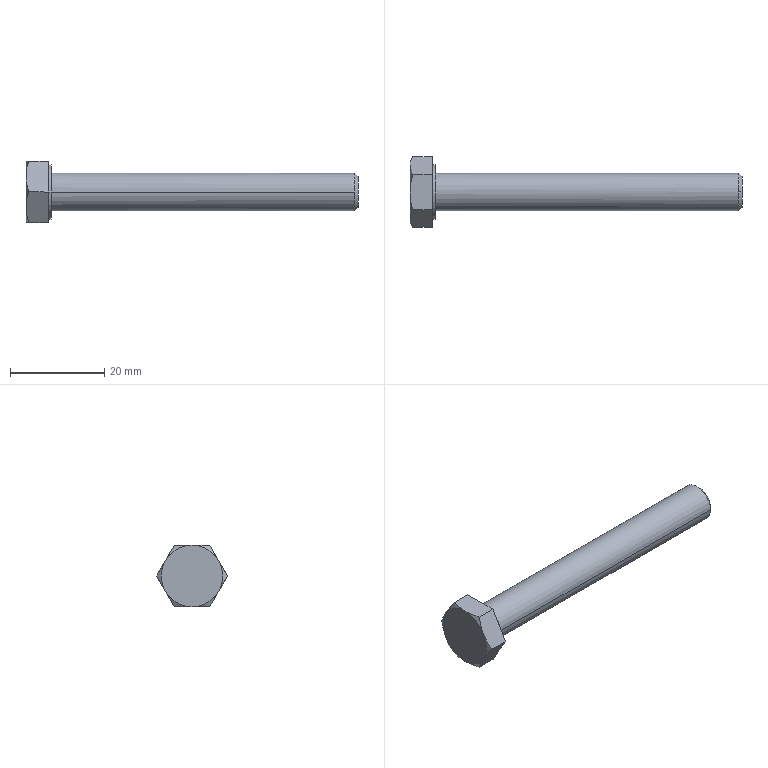Part | STEP file | DIN 931-1 - M8 x 65 | 1 solid | 22 faces | box 70.3 x 15.011 x 13 mm | volume 4009 mm3 | plane 10 | cone 8 | cylinder 4 | commonest cylinder face diameters 8 x2 11.6 x2